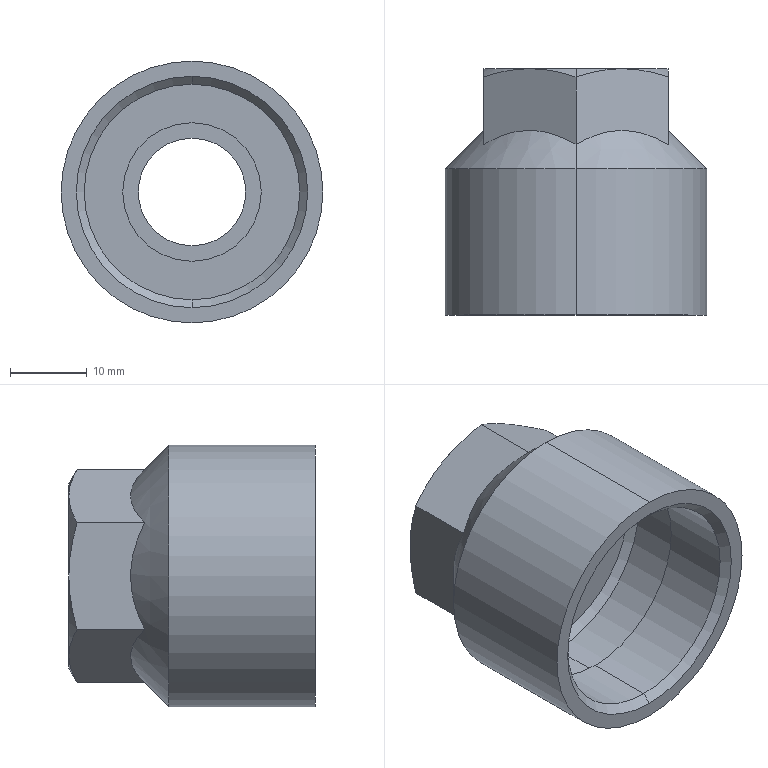Part | SolidWorks | features ICE 6, Chamfer 2, Extrusion 1, HoleWzd 1 | 1 solid | 36 faces | box 34 x 32 x 34 mm | volume 9791 mm3 | cone 15 | plane 11 | cylinder 10 | commonest cylinder face diameters 14 x2 18 x2 28 x2 30 x2 34 x2
STEP:
#1=CARTESIAN_POINT('',(0.,8.,12.));
#2=VERTEX_POINT('',#1);
#3=CARTESIAN_POINT('',(6.,8.,10.392));
#4=VERTEX_POINT('',#3);
#5=CARTESIAN_POINT('',(0.,8.,0.));
#6=DIRECTION('',(0.,1.,0.));
#7=DIRECTION('',(0.,0.,1.));
#8=AXIS2_PLACEMENT_3D('',#5,#6,#7);
#9=CIRCLE('',#8,12.);
#10=EDGE_CURVE('',#2,#4,#9,.T.);
#11=ORIENTED_EDGE('',*,*,#10,.F.);
#12=CARTESIAN_POINT('',(0.,6.928,13.856));
#13=VERTEX_POINT('',#12);
#14=CARTESIAN_POINT('',(0.,8.,12.));
#15=DIRECTION('',(0.,-0.5,0.866));
#16=VECTOR('',#15,1000.);
#17=LINE('',#14,#16);
#18=EDGE_CURVE('',#2,#13,#17,.T.);
#19=ORIENTED_EDGE('',*,*,#18,.T.);
#20=CARTESIAN_POINT('',(0.,6.928,13.856));
#21=CARTESIAN_POINT('',(0.9815,7.255,13.29));
#22=CARTESIAN_POINT('',(1.97,7.525,12.719));
#23=CARTESIAN_POINT('',(3.968,7.898,11.565));
#24=CARTESIAN_POINT('',(4.978,8.,10.982));
#25=CARTESIAN_POINT('',(6.,8.,10.392));
#26=B_SPLINE_CURVE_WITH_KNOTS('',3,(#20,#21,#22,#23,#24,#25),.UNSPECIFIED.,.F.,.F.,(4,2,4),(0.000000238,0.003505,0.00701),.UNSPECIFIED.);
#27=EDGE_CURVE('',#13,#4,#26,.T.);
#28=ORIENTED_EDGE('',*,*,#27,.T.);
#29=EDGE_LOOP('',(#11,#19,#28));
#30=FACE_OUTER_BOUND('',#29,.T.);
#31=CARTESIAN_POINT('',(0.,8.,0.));
#32=DIRECTION('',(0.,-1.,0.));
#33=DIRECTION('',(0.,0.,1.));
#34=AXIS2_PLACEMENT_3D('',#31,#32,#33);
#35=CONICAL_SURFACE('',#34,12.,1.047);
#36=ADVANCED_FACE('',(#30),#35,.T.);
#37=CARTESIAN_POINT('',(0.,-1.856,13.856));
#38=VERTEX_POINT('',#37);
#39=CARTESIAN_POINT('',(12.,-1.856,6.928));
#40=VERTEX_POINT('',#39);
#41=CARTESIAN_POINT('',(0.,-1.856,13.856));
#42=CARTESIAN_POINT('',(0.9376,-1.315,13.315));
#43=CARTESIAN_POINT('',(1.896,-0.8548,12.762));
#44=CARTESIAN_POINT('',(3.386,-0.3616,11.902));
#45=CARTESIAN_POINT('',(3.891,-0.2304,11.61));
#46=CARTESIAN_POINT('',(4.923,-0.04992,11.014));
#47=CARTESIAN_POINT('',(5.454,-0.001312,10.707));
#48=CARTESIAN_POINT('',(7.025,0.002543,9.8));
#49=CARTESIAN_POINT('',(8.055,-0.1806,9.206));
#50=CARTESIAN_POINT('',(10.086,-0.845,8.033));
#51=CARTESIAN_POINT('',(11.057,-1.312,7.473));
#52=CARTESIAN_POINT('',(12.,-1.856,6.928));
#53=B_SPLINE_CURVE_WITH_KNOTS('',3,(#41,#42,#43,#44,#45,#46,#47,#48,#49,#50,#51,#52),.UNSPECIFIED.,.F.,.F.,(4,2,2,2,2,4),(0.,0.003578,0.005367,0.007157,0.01073,0.01431),.UNSPECIFIED.);
#54=EDGE_CURVE('',#38,#40,#53,.T.);
#55=ORIENTED_EDGE('',*,*,#54,.F.);
#56=CARTESIAN_POINT('',(0.,-5.,17.));
#57=VERTEX_POINT('',#56);
#58=CARTESIAN_POINT('',(0.,-5.,17.));
#59=DIRECTION('',(0.,-0.7071,0.7071));
#60=VECTOR('',#59,1000.);
#61=LINE('',#58,#60);
#62=EDGE_CURVE('',#38,#57,#61,.T.);
#63=ORIENTED_EDGE('',*,*,#62,.T.);
#64=CARTESIAN_POINT('',(0.,-5.,-17.));
#65=VERTEX_POINT('',#64);
#66=CARTESIAN_POINT('',(0.,-5.,0.));
#67=DIRECTION('',(0.,-1.,0.));
#68=DIRECTION('',(0.,0.,-1.));
#69=AXIS2_PLACEMENT_3D('',#66,#67,#68);
#70=CIRCLE('',#69,17.);
#71=EDGE_CURVE('',#65,#57,#70,.T.);
#72=ORIENTED_EDGE('',*,*,#71,.F.);
#73=CARTESIAN_POINT('',(0.,-1.856,-13.856));
#74=VERTEX_POINT('',#73);
#75=CARTESIAN_POINT('',(0.,-5.,-17.));
#76=DIRECTION('',(0.,-0.7071,-0.7071));
#77=VECTOR('',#76,1000.);
#78=LINE('',#75,#77);
#79=EDGE_CURVE('',#74,#65,#78,.T.);
#80=ORIENTED_EDGE('',*,*,#79,.F.);
#81=CARTESIAN_POINT('',(12.,-1.856,-6.928));
#82=VERTEX_POINT('',#81);
#83=CARTESIAN_POINT('',(12.,-1.856,-6.928));
#84=CARTESIAN_POINT('',(11.062,-1.315,-7.47));
#85=CARTESIAN_POINT('',(10.104,-0.8548,-8.023));
#86=CARTESIAN_POINT('',(8.614,-0.3616,-8.883));
#87=CARTESIAN_POINT('',(8.109,-0.2304,-9.175));
#88=CARTESIAN_POINT('',(7.077,-0.04992,-9.77));
#89=CARTESIAN_POINT('',(6.546,-0.001312,-10.077));
#90=CARTESIAN_POINT('',(4.975,0.002543,-10.984));
#91=CARTESIAN_POINT('',(3.945,-0.1806,-11.579));
#92=CARTESIAN_POINT('',(1.914,-0.845,-12.751));
#93=CARTESIAN_POINT('',(0.9431,-1.312,-13.312));
#94=CARTESIAN_POINT('',(0.,-1.856,-13.856));
#95=B_SPLINE_CURVE_WITH_KNOTS('',3,(#83,#84,#85,#86,#87,#88,#89,#90,#91,#92,#93,#94),.UNSPECIFIED.,.F.,.F.,(4,2,2,2,2,4),(0.,0.003578,0.005367,0.007157,0.01073,0.01431),.UNSPECIFIED.);
#96=EDGE_CURVE('',#82,#74,#95,.T.);
#97=ORIENTED_EDGE('',*,*,#96,.F.);
#98=CARTESIAN_POINT('',(12.,-1.856,6.928));
#99=CARTESIAN_POINT('',(12.,-1.315,5.846));
#100=CARTESIAN_POINT('',(12.,-0.8548,4.739));
#101=CARTESIAN_POINT('',(12.,-0.3616,3.019));
#102=CARTESIAN_POINT('',(12.,-0.2304,2.435));
#103=CARTESIAN_POINT('',(12.,-0.04992,1.244));
#104=CARTESIAN_POINT('',(12.,-0.001312,0.6303));
#105=CARTESIAN_POINT('',(12.,0.002543,-1.184));
#106=CARTESIAN_POINT('',(12.,-0.1806,-2.373));
#107=CARTESIAN_POINT('',(12.,-0.845,-4.718));
#108=CARTESIAN_POINT('',(12.,-1.312,-5.839));
#109=CARTESIAN_POINT('',(12.,-1.856,-6.928));
#110=B_SPLINE_CURVE_WITH_KNOTS('',3,(#98,#99,#100,#101,#102,#103,#104,#105,#106,#107,#108,#109),.UNSPECIFIED.,.F.,.F.,(4,2,2,2,2,4),(0.,0.003578,0.005367,0.007157,0.01073,0.01431),.UNSPECIFIED.);
#111=EDGE_CURVE('',#40,#82,#110,.T.);
#112=ORIENTED_EDGE('',*,*,#111,.F.);
#113=EDGE_LOOP('',(#55,#63,#72,#80,#97,#112));
#114=FACE_OUTER_BOUND('',#113,.T.);
#115=CARTESIAN_POINT('',(0.,-5.,0.));
#116=DIRECTION('',(0.,-1.,0.));
#117=DIRECTION('',(0.,0.,-1.));
#118=AXIS2_PLACEMENT_3D('',#115,#116,#117);
#119=CONICAL_SURFACE('',#118,17.,0.7854);
#120=ADVANCED_FACE('',(#114),#119,.T.);
#121=CARTESIAN_POINT('',(0.,7.,-7.));
#122=VERTEX_POINT('',#121);
#123=CARTESIAN_POINT('',(0.,7.,7.));
#124=VERTEX_POINT('',#123);
#125=CARTESIAN_POINT('',(0.,7.,0.));
#126=DIRECTION('',(0.,1.,0.));
#127=DIRECTION('',(0.,0.,1.));
#128=AXIS2_PLACEMENT_3D('',#125,#126,#127);
#129=CIRCLE('',#128,7.);
#130=EDGE_CURVE('',#122,#124,#129,.T.);
#131=ORIENTED_EDGE('',*,*,#130,.F.);
#132=CARTESIAN_POINT('',(0.,8.,-8.));
#133=VERTEX_POINT('',#132);
#134=CARTESIAN_POINT('',(0.,7.,-7.));
#135=DIRECTION('',(0.,0.7071,-0.7071));
#136=VECTOR('',#135,1000.);
#137=LINE('',#134,#136);
#138=EDGE_CURVE('',#122,#133,#137,.T.);
#139=ORIENTED_EDGE('',*,*,#138,.T.);
#140=CARTESIAN_POINT('',(0.,8.,8.));
#141=VERTEX_POINT('',#140);
#142=CARTESIAN_POINT('',(0.,8.,0.));
#143=DIRECTION('',(0.,-1.,0.));
#144=DIRECTION('',(0.,0.,1.));
#145=AXIS2_PLACEMENT_3D('',#142,#143,#144);
#146=CIRCLE('',#145,8.);
#147=EDGE_CURVE('',#141,#133,#146,.T.);
#148=ORIENTED_EDGE('',*,*,#147,.F.);
#149=CARTESIAN_POINT('',(0.,7.,7.));
#150=DIRECTION('',(0.,0.7071,0.7071));
#151=VECTOR('',#150,1000.);
#152=LINE('',#149,#151);
#153=EDGE_CURVE('',#124,#141,#152,.T.);
#154=ORIENTED_EDGE('',*,*,#153,.F.);
#155=EDGE_LOOP('',(#131,#139,#148,#154));
#156=FACE_OUTER_BOUND('',#155,.T.);
#157=CARTESIAN_POINT('',(0.,7.,0.));
#158=DIRECTION('',(0.,1.,0.));
#159=DIRECTION('',(0.,0.,1.));
#160=AXIS2_PLACEMENT_3D('',#157,#158,#159);
#161=CONICAL_SURFACE('',#160,7.,0.7854);
#162=ADVANCED_FACE('',(#156),#161,.F.);
#163=CARTESIAN_POINT('',(0.,-6.,-14.));
#164=VERTEX_POINT('',#163);
#165=CARTESIAN_POINT('',(0.,-6.,14.));
#166=VERTEX_POINT('',#165);
#167=CARTESIAN_POINT('',(0.,-6.,0.));
#168=DIRECTION('',(0.,1.,0.));
#169=DIRECTION('',(0.,0.,1.));
#170=AXIS2_PLACEMENT_3D('',#167,#168,#169);
#171=CIRCLE('',#170,14.);
#172=EDGE_CURVE('',#164,#166,#171,.T.);
#173=ORIENTED_EDGE('',*,*,#172,.T.);
#174=CARTESIAN_POINT('',(0.,-7.,15.));
#175=VERTEX_POINT('',#174);
#176=CARTESIAN_POINT('',(0.,-7.,15.));
#177=DIRECTION('',(0.,-0.7071,0.7071));
#178=VECTOR('',#177,1000.);
#179=LINE('',#176,#178);
#180=EDGE_CURVE('',#166,#175,#179,.T.);
#181=ORIENTED_EDGE('',*,*,#180,.T.);
#182=CARTESIAN_POINT('',(0.,-7.,-15.));
#183=VERTEX_POINT('',#182);
#184=CARTESIAN_POINT('',(0.,-7.,0.));
#185=DIRECTION('',(0.,1.,0.));
#186=DIRECTION('',(0.,0.,1.));
#187=AXIS2_PLACEMENT_3D('',#184,#185,#186);
#188=CIRCLE('',#187,15.);
#189=EDGE_CURVE('',#183,#175,#188,.T.);
#190=ORIENTED_EDGE('',*,*,#189,.F.);
#191=CARTESIAN_POINT('',(0.,-7.,-15.));
#192=DIRECTION('',(0.,-0.7071,-0.7071));
#193=VECTOR('',#192,1000.);
#194=LINE('',#191,#193);
#195=EDGE_CURVE('',#164,#183,#194,.T.);
#196=ORIENTED_EDGE('',*,*,#195,.F.);
#197=EDGE_LOOP('',(#173,#181,#190,#196));
#198=FACE_OUTER_BOUND('',#197,.T.);
#199=CARTESIAN_POINT('',(0.,-7.,0.));
#200=DIRECTION('',(0.,-1.,0.));
#201=DIRECTION('',(0.,0.,-1.));
#202=AXIS2_PLACEMENT_3D('',#199,#200,#201);
#203=CONICAL_SURFACE('',#202,15.,0.7854);
#204=ADVANCED_FACE('',(#198),#203,.F.);
#205=CARTESIAN_POINT('',(0.,-22.975,14.));
#206=VERTEX_POINT('',#205);
#207=CARTESIAN_POINT('',(0.,-22.975,-14.));
#208=VERTEX_POINT('',#207);
#209=CARTESIAN_POINT('',(0.,-22.975,0.));
#210=DIRECTION('',(0.,-1.,0.));
#211=DIRECTION('',(0.,0.,-1.));
#212=AXIS2_PLACEMENT_3D('',#209,#210,#211);
#213=CIRCLE('',#212,14.);
#214=EDGE_CURVE('',#206,#208,#213,.T.);
#215=ORIENTED_EDGE('',*,*,#214,.F.);
#216=CARTESIAN_POINT('',(0.,-24.,15.025));
#217=VERTEX_POINT('',#216);
#218=CARTESIAN_POINT('',(0.,-24.,15.025));
#219=DIRECTION('',(0.,-0.7071,0.7071));
#220=VECTOR('',#219,1000.);
#221=LINE('',#218,#220);
#222=EDGE_CURVE('',#206,#217,#221,.T.);
#223=ORIENTED_EDGE('',*,*,#222,.T.);
#224=CARTESIAN_POINT('',(0.,-24.,-15.025));
#225=VERTEX_POINT('',#224);
#226=CARTESIAN_POINT('',(0.,-24.,0.));
#227=DIRECTION('',(0.,-1.,0.));
#228=DIRECTION('',(0.,0.,-1.));
#229=AXIS2_PLACEMENT_3D('',#226,#227,#228);
#230=CIRCLE('',#229,15.025);
#231=EDGE_CURVE('',#217,#225,#230,.T.);
#232=ORIENTED_EDGE('',*,*,#231,.T.);
#233=CARTESIAN_POINT('',(0.,-24.,-15.025));
#234=DIRECTION('',(0.,-0.7071,-0.7071));
#235=VECTOR('',#234,1000.);
#236=LINE('',#233,#235);
#237=EDGE_CURVE('',#208,#225,#236,.T.);
#238=ORIENTED_EDGE('',*,*,#237,.F.);
#239=EDGE_LOOP('',(#215,#223,#232,#238));
#240=FACE_OUTER_BOUND('',#239,.T.);
#241=CARTESIAN_POINT('',(0.,-24.,0.));
#242=DIRECTION('',(0.,-1.,0.));
#243=DIRECTION('',(0.,0.,-1.));
#244=AXIS2_PLACEMENT_3D('',#241,#242,#243);
#245=CONICAL_SURFACE('',#244,15.025,0.7854);
#246=ADVANCED_FACE('',(#240),#245,.F.);
#247=CARTESIAN_POINT('',(0.,-14.,14.));
#248=VERTEX_POINT('',#247);
#249=CARTESIAN_POINT('',(0.,-14.,-14.));
#250=VERTEX_POINT('',#249);
#251=CARTESIAN_POINT('',(0.,-14.,0.));
#252=DIRECTION('',(0.,-1.,0.));
#253=DIRECTION('',(0.,0.,-1.));
#254=AXIS2_PLACEMENT_3D('',#251,#252,#253);
#255=CIRCLE('',#254,14.);
#256=EDGE_CURVE('',#248,#250,#255,.T.);
#257=ORIENTED_EDGE('',*,*,#256,.F.);
#258=CARTESIAN_POINT('',(0.,-24.,14.));
#259=DIRECTION('',(0.,-1.,0.));
#260=VECTOR('',#259,1000.);
#261=LINE('',#258,#260);
#262=EDGE_CURVE('',#248,#206,#261,.T.);
#263=ORIENTED_EDGE('',*,*,#262,.T.);
#264=ORIENTED_EDGE('',*,*,#214,.T.);
#265=CARTESIAN_POINT('',(0.,-24.,-14.));
#266=DIRECTION('',(0.,-1.,0.));
#267=VECTOR('',#266,1000.);
#268=LINE('',#265,#267);
#269=EDGE_CURVE('',#250,#208,#268,.T.);
#270=ORIENTED_EDGE('',*,*,#269,.F.);
#271=EDGE_LOOP('',(#257,#263,#264,#270));
#272=FACE_OUTER_BOUND('',#271,.T.);
#273=CARTESIAN_POINT('',(0.,-24.,0.));
#274=DIRECTION('',(0.,-1.,0.));
#275=DIRECTION('',(0.,0.,-1.));
#276=AXIS2_PLACEMENT_3D('',#273,#274,#275);
#277=CYLINDRICAL_SURFACE('',#276,14.);
#278=ADVANCED_FACE('',(#272),#277,.F.);
#279=CARTESIAN_POINT('',(0.,-14.,-15.));
#280=VERTEX_POINT('',#279);
#281=CARTESIAN_POINT('',(0.,-14.,15.));
#282=VERTEX_POINT('',#281);
#283=CARTESIAN_POINT('',(0.,-14.,0.));
#284=DIRECTION('',(0.,1.,0.));
#285=DIRECTION('',(0.,0.,1.));
#286=AXIS2_PLACEMENT_3D('',#283,#284,#285);
#287=CIRCLE('',#286,15.);
#288=EDGE_CURVE('',#280,#282,#287,.T.);
#289=ORIENTED_EDGE('',*,*,#288,.F.);
#290=CARTESIAN_POINT('',(0.,-14.,-15.));
#291=DIRECTION('',(0.,1.,0.));
#292=VECTOR('',#291,1000.);
#293=LINE('',#290,#292);
#294=EDGE_CURVE('',#280,#183,#293,.T.);
#295=ORIENTED_EDGE('',*,*,#294,.T.);
#296=ORIENTED_EDGE('',*,*,#189,.T.);
#297=CARTESIAN_POINT('',(0.,-14.,15.));
#298=DIRECTION('',(0.,1.,0.));
#299=VECTOR('',#298,1000.);
#300=LINE('',#297,#299);
#301=EDGE_CURVE('',#282,#175,#300,.T.);
#302=ORIENTED_EDGE('',*,*,#301,.F.);
#303=EDGE_LOOP('',(#289,#295,#296,#302));
#304=FACE_OUTER_BOUND('',#303,.T.);
#305=CARTESIAN_POINT('',(0.,-14.,0.));
#306=DIRECTION('',(0.,1.,0.));
#307=DIRECTION('',(0.,0.,1.));
#308=AXIS2_PLACEMENT_3D('',#305,#306,#307);
#309=CYLINDRICAL_SURFACE('',#308,15.);
#310=ADVANCED_FACE('',(#304),#309,.F.);
#311=CARTESIAN_POINT('',(0.,-6.,-9.));
#312=VERTEX_POINT('',#311);
#313=CARTESIAN_POINT('',(0.,-6.,9.));
#314=VERTEX_POINT('',#313);
#315=CARTESIAN_POINT('',(0.,-6.,0.));
#316=DIRECTION('',(0.,1.,0.));
#317=DIRECTION('',(0.,0.,1.));
#318=AXIS2_PLACEMENT_3D('',#315,#316,#317);
#319=CIRCLE('',#318,9.);
#320=EDGE_CURVE('',#312,#314,#319,.T.);
#321=ORIENTED_EDGE('',*,*,#320,.F.);
#322=CARTESIAN_POINT('',(0.,2.,-9.));
#323=VERTEX_POINT('',#322);
#324=CARTESIAN_POINT('',(0.,-6.,-9.));
#325=DIRECTION('',(0.,1.,0.));
#326=VECTOR('',#325,1000.);
#327=LINE('',#324,#326);
#328=EDGE_CURVE('',#312,#323,#327,.T.);
#329=ORIENTED_EDGE('',*,*,#328,.T.);
#330=CARTESIAN_POINT('',(0.,2.,9.));
#331=VERTEX_POINT('',#330);
#332=CARTESIAN_POINT('',(0.,2.,0.));
#333=DIRECTION('',(0.,1.,0.));
#334=DIRECTION('',(0.,0.,1.));
#335=AXIS2_PLACEMENT_3D('',#332,#333,#334);
#336=CIRCLE('',#335,9.);
#337=EDGE_CURVE('',#323,#331,#336,.T.);
#338=ORIENTED_EDGE('',*,*,#337,.T.);
#339=CARTESIAN_POINT('',(0.,-6.,9.));
#340=DIRECTION('',(0.,1.,0.));
#341=VECTOR('',#340,1000.);
#342=LINE('',#339,#341);
#343=EDGE_CURVE('',#314,#331,#342,.T.);
#344=ORIENTED_EDGE('',*,*,#343,.F.);
#345=EDGE_LOOP('',(#321,#329,#338,#344));
#346=FACE_OUTER_BOUND('',#345,.T.);
#347=CARTESIAN_POINT('',(0.,-6.,0.));
#348=DIRECTION('',(0.,1.,0.));
#349=DIRECTION('',(0.,0.,1.));
#350=AXIS2_PLACEMENT_3D('',#347,#348,#349);
#351=CYLINDRICAL_SURFACE('',#350,9.);
#352=ADVANCED_FACE('',(#346),#351,.F.);
#353=CARTESIAN_POINT('',(0.,2.,-7.));
#354=VERTEX_POINT('',#353);
#355=CARTESIAN_POINT('',(0.,2.,7.));
#356=VERTEX_POINT('',#355);
#357=CARTESIAN_POINT('',(0.,2.,0.));
#358=DIRECTION('',(0.,1.,0.));
#359=DIRECTION('',(0.,0.,1.));
#360=AXIS2_PLACEMENT_3D('',#357,#358,#359);
#361=CIRCLE('',#360,7.);
#362=EDGE_CURVE('',#354,#356,#361,.T.);
#363=ORIENTED_EDGE('',*,*,#362,.F.);
#364=CARTESIAN_POINT('',(0.,2.,-7.));
#365=DIRECTION('',(0.,1.,0.));
#366=VECTOR('',#365,1000.);
#367=LINE('',#364,#366);
#368=EDGE_CURVE('',#354,#122,#367,.T.);
#369=ORIENTED_EDGE('',*,*,#368,.T.);
#370=ORIENTED_EDGE('',*,*,#130,.T.);
#371=CARTESIAN_POINT('',(0.,2.,7.));
#372=DIRECTION('',(0.,1.,0.));
#373=VECTOR('',#372,1000.);
#374=LINE('',#371,#373);
#375=EDGE_CURVE('',#356,#124,#374,.T.);
#376=ORIENTED_EDGE('',*,*,#375,.F.);
#377=EDGE_LOOP('',(#363,#369,#370,#376));
#378=FACE_OUTER_BOUND('',#377,.T.);
#379=CARTESIAN_POINT('',(0.,2.,0.));
#380=DIRECTION('',(0.,1.,0.));
#381=DIRECTION('',(0.,0.,1.));
#382=AXIS2_PLACEMENT_3D('',#379,#380,#381);
#383=CYLINDRICAL_SURFACE('',#382,7.);
#384=ADVANCED_FACE('',(#378),#383,.F.);
#385=CARTESIAN_POINT('',(0.,-24.,-17.));
#386=VERTEX_POINT('',#385);
#387=CARTESIAN_POINT('',(0.,-24.,17.));
#388=VERTEX_POINT('',#387);
#389=CARTESIAN_POINT('',(0.,-24.,0.));
#390=DIRECTION('',(0.,-1.,0.));
#391=DIRECTION('',(0.,0.,-1.));
#392=AXIS2_PLACEMENT_3D('',#389,#390,#391);
#393=CIRCLE('',#392,17.);
#394=EDGE_CURVE('',#386,#388,#393,.T.);
#395=ORIENTED_EDGE('',*,*,#394,.F.);
#396=CARTESIAN_POINT('',(0.,-24.,-17.));
#397=DIRECTION('',(0.,1.,0.));
#398=VECTOR('',#397,1000.);
#399=LINE('',#396,#398);
#400=EDGE_CURVE('',#386,#65,#399,.T.);
#401=ORIENTED_EDGE('',*,*,#400,.T.);
#402=ORIENTED_EDGE('',*,*,#71,.T.);
#403=CARTESIAN_POINT('',(0.,-24.,17.));
#404=DIRECTION('',(0.,1.,0.));
#405=VECTOR('',#404,1000.);
#406=LINE('',#403,#405);
#407=EDGE_CURVE('',#388,#57,#406,.T.);
#408=ORIENTED_EDGE('',*,*,#407,.F.);
#409=EDGE_LOOP('',(#395,#401,#402,#408));
#410=FACE_OUTER_BOUND('',#409,.T.);
#411=CARTESIAN_POINT('',(0.,-24.,0.));
#412=DIRECTION('',(0.,1.,0.));
#413=DIRECTION('',(0.,0.,1.));
#414=AXIS2_PLACEMENT_3D('',#411,#412,#413);
#415=CYLINDRICAL_SURFACE('',#414,17.);
#416=ADVANCED_FACE('',(#410),#415,.T.);
#417=CARTESIAN_POINT('',(12.,6.928,-6.928));
#418=VERTEX_POINT('',#417);
#419=CARTESIAN_POINT('',(6.,8.,-10.392));
#420=VERTEX_POINT('',#419);
#421=CARTESIAN_POINT('',(12.,6.928,-6.928));
#422=CARTESIAN_POINT('',(11.018,7.255,-7.495));
#423=CARTESIAN_POINT('',(10.03,7.525,-8.066));
#424=CARTESIAN_POINT('',(8.032,7.898,-9.219));
#425=CARTESIAN_POINT('',(7.022,8.,-9.802));
#426=CARTESIAN_POINT('',(6.,8.,-10.392));
#427=B_SPLINE_CURVE_WITH_KNOTS('',3,(#421,#422,#423,#424,#425,#426),.UNSPECIFIED.,.F.,.F.,(4,2,4),(0.000000238,0.003505,0.00701),.UNSPECIFIED.);
#428=EDGE_CURVE('',#418,#420,#427,.T.);
#429=ORIENTED_EDGE('',*,*,#428,.F.);
#430=CARTESIAN_POINT('',(12.,8.,-6.928));
#431=DIRECTION('',(0.,-1.,0.));
#432=VECTOR('',#431,1000.);
#433=LINE('',#430,#432);
#434=EDGE_CURVE('',#418,#82,#433,.T.);
#435=ORIENTED_EDGE('',*,*,#434,.T.);
#436=ORIENTED_EDGE('',*,*,#96,.T.);
#437=CARTESIAN_POINT('',(0.,6.928,-13.856));
#438=VERTEX_POINT('',#437);
#439=CARTESIAN_POINT('',(0.,8.,-13.856));
#440=DIRECTION('',(0.,-1.,0.));
#441=VECTOR('',#440,1000.);
#442=LINE('',#439,#441);
#443=EDGE_CURVE('',#438,#74,#442,.T.);
#444=ORIENTED_EDGE('',*,*,#443,.F.);
#445=CARTESIAN_POINT('',(6.,8.,-10.392));
#446=CARTESIAN_POINT('',(5.491,8.,-10.686));
#447=CARTESIAN_POINT('',(4.979,7.975,-10.982));
#448=CARTESIAN_POINT('',(3.967,7.877,-11.566));
#449=CARTESIAN_POINT('',(3.465,7.804,-11.856));
#450=CARTESIAN_POINT('',(1.966,7.524,-12.721));
#451=CARTESIAN_POINT('',(0.9791,7.255,-13.291));
#452=CARTESIAN_POINT('',(0.,6.928,-13.856));
#453=B_SPLINE_CURVE_WITH_KNOTS('',3,(#445,#446,#447,#448,#449,#450,#451,#452),.UNSPECIFIED.,.F.,.F.,(4,2,2,4),(0.00701,0.008756,0.0105,0.01399),.UNSPECIFIED.);
#454=EDGE_CURVE('',#420,#438,#453,.T.);
#455=ORIENTED_EDGE('',*,*,#454,.F.);
#456=EDGE_LOOP('',(#429,#435,#436,#444,#455));
#457=FACE_OUTER_BOUND('',#456,.T.);
#458=CARTESIAN_POINT('',(12.,8.,-6.928));
#459=DIRECTION('',(-0.5,0.,0.866));
#460=DIRECTION('',(0.866,0.,0.5));
#461=AXIS2_PLACEMENT_3D('',#458,#459,#460);
#462=PLANE('',#461);
#463=ADVANCED_FACE('',(#457),#462,.F.);
#464=CARTESIAN_POINT('',(-6.,8.,-10.392));
#465=VERTEX_POINT('',#464);
#466=CARTESIAN_POINT('',(0.,6.928,-13.856));
#467=CARTESIAN_POINT('',(-0.9815,7.255,-13.29));
#468=CARTESIAN_POINT('',(-1.97,7.525,-12.719));
#469=CARTESIAN_POINT('',(-3.968,7.898,-11.565));
#470=CARTESIAN_POINT('',(-4.978,8.,-10.982));
#471=CARTESIAN_POINT('',(-6.,8.,-10.392));
#472=B_SPLINE_CURVE_WITH_KNOTS('',3,(#466,#467,#468,#469,#470,#471),.UNSPECIFIED.,.F.,.F.,(4,2,4),(0.000000238,0.003505,0.00701),.UNSPECIFIED.);
#473=EDGE_CURVE('',#438,#465,#472,.T.);
#474=ORIENTED_EDGE('',*,*,#473,.F.);
#475=ORIENTED_EDGE('',*,*,#443,.T.);
#476=CARTESIAN_POINT('',(-12.,-1.856,-6.928));
#477=VERTEX_POINT('',#476);
#478=CARTESIAN_POINT('',(0.,-1.856,-13.856));
#479=CARTESIAN_POINT('',(-0.9376,-1.315,-13.315));
#480=CARTESIAN_POINT('',(-1.896,-0.8549,-12.762));
#481=CARTESIAN_POINT('',(-3.386,-0.3617,-11.902));
#482=CARTESIAN_POINT('',(-3.891,-0.2305,-11.61));
#483=CARTESIAN_POINT('',(-4.923,-0.04994,-11.014));
#484=CARTESIAN_POINT('',(-5.454,-0.001324,-10.708));
#485=CARTESIAN_POINT('',(-7.025,0.002566,-9.8));
#486=CARTESIAN_POINT('',(-8.055,-0.1806,-9.206));
#487=CARTESIAN_POINT('',(-10.086,-0.8452,-8.033));
#488=CARTESIAN_POINT('',(-11.057,-1.312,-7.473));
#489=CARTESIAN_POINT('',(-12.,-1.856,-6.928));
#490=B_SPLINE_CURVE_WITH_KNOTS('',3,(#478,#479,#480,#481,#482,#483,#484,#485,#486,#487,#488,#489),.UNSPECIFIED.,.F.,.F.,(4,2,2,2,2,4),(-0.01096,-0.007318,-0.005498,-0.003678,-0.00003841,0.003601),.UNSPECIFIED.);
#491=EDGE_CURVE('',#74,#477,#490,.T.);
#492=ORIENTED_EDGE('',*,*,#491,.T.);
#493=CARTESIAN_POINT('',(-12.,6.928,-6.928));
#494=VERTEX_POINT('',#493);
#495=CARTESIAN_POINT('',(-12.,8.,-6.928));
#496=DIRECTION('',(0.,-1.,0.));
#497=VECTOR('',#496,1000.);
#498=LINE('',#495,#497);
#499=EDGE_CURVE('',#494,#477,#498,.T.);
#500=ORIENTED_EDGE('',*,*,#499,.F.);
#501=CARTESIAN_POINT('',(-6.,8.,-10.392));
#502=CARTESIAN_POINT('',(-6.509,8.,-10.098));
#503=CARTESIAN_POINT('',(-7.021,7.975,-9.803));
#504=CARTESIAN_POINT('',(-8.033,7.877,-9.219));
#505=CARTESIAN_POINT('',(-8.535,7.804,-8.929));
#506=CARTESIAN_POINT('',(-10.034,7.524,-8.063));
#507=CARTESIAN_POINT('',(-11.021,7.255,-7.493));
#508=CARTESIAN_POINT('',(-12.,6.928,-6.928));
#509=B_SPLINE_CURVE_WITH_KNOTS('',3,(#501,#502,#503,#504,#505,#506,#507,#508),.UNSPECIFIED.,.F.,.F.,(4,2,2,4),(0.00701,0.008756,0.0105,0.01399),.UNSPECIFIED.);
#510=EDGE_CURVE('',#465,#494,#509,.T.);
#511=ORIENTED_EDGE('',*,*,#510,.F.);
#512=EDGE_LOOP('',(#474,#475,#492,#500,#511));
#513=FACE_OUTER_BOUND('',#512,.T.);
#514=CARTESIAN_POINT('',(0.,8.,-13.856));
#515=DIRECTION('',(0.5,0.,0.866));
#516=DIRECTION('',(0.866,0.,-0.5));
#517=AXIS2_PLACEMENT_3D('',#514,#515,#516);
#518=PLANE('',#517);
#519=ADVANCED_FACE('',(#513),#518,.F.);
#520=CARTESIAN_POINT('',(-12.,8.,0.));
#521=VERTEX_POINT('',#520);
#522=CARTESIAN_POINT('',(-12.,6.928,-6.928));
#523=CARTESIAN_POINT('',(-12.,7.254,-5.8));
#524=CARTESIAN_POINT('',(-12.,7.523,-4.662));
#525=CARTESIAN_POINT('',(-12.,7.897,-2.356));
#526=CARTESIAN_POINT('',(-12.,8.,-1.187));
#527=CARTESIAN_POINT('',(-12.,8.,0.));
#528=B_SPLINE_CURVE_WITH_KNOTS('',3,(#522,#523,#524,#525,#526,#527),.UNSPECIFIED.,.F.,.F.,(4,2,4),(0.01541,0.01893,0.02245),.UNSPECIFIED.);
#529=EDGE_CURVE('',#494,#521,#528,.T.);
#530=ORIENTED_EDGE('',*,*,#529,.F.);
#531=ORIENTED_EDGE('',*,*,#499,.T.);
#532=CARTESIAN_POINT('',(-12.,-1.856,6.928));
#533=VERTEX_POINT('',#532);
#534=CARTESIAN_POINT('',(-12.,-1.856,-6.928));
#535=CARTESIAN_POINT('',(-12.,-1.315,-5.846));
#536=CARTESIAN_POINT('',(-12.,-0.8548,-4.739));
#537=CARTESIAN_POINT('',(-12.,-0.3616,-3.019));
#538=CARTESIAN_POINT('',(-12.,-0.2304,-2.435));
#539=CARTESIAN_POINT('',(-12.,-0.04992,-1.244));
#540=CARTESIAN_POINT('',(-12.,-0.001312,-0.6303));
#541=CARTESIAN_POINT('',(-12.,0.002543,1.184));
#542=CARTESIAN_POINT('',(-12.,-0.1806,2.373));
#543=CARTESIAN_POINT('',(-12.,-0.845,4.718));
#544=CARTESIAN_POINT('',(-12.,-1.312,5.839));
#545=CARTESIAN_POINT('',(-12.,-1.856,6.928));
#546=B_SPLINE_CURVE_WITH_KNOTS('',3,(#534,#535,#536,#537,#538,#539,#540,#541,#542,#543,#544,#545),.UNSPECIFIED.,.F.,.F.,(4,2,2,2,2,4),(0.,0.003578,0.005367,0.007157,0.01073,0.01431),.UNSPECIFIED.);
#547=EDGE_CURVE('',#477,#533,#546,.T.);
#548=ORIENTED_EDGE('',*,*,#547,.T.);
#549=CARTESIAN_POINT('',(-12.,6.928,6.928));
#550=VERTEX_POINT('',#549);
#551=CARTESIAN_POINT('',(-12.,8.,6.928));
#552=DIRECTION('',(0.,-1.,0.));
#553=VECTOR('',#552,1000.);
#554=LINE('',#551,#553);
#555=EDGE_CURVE('',#550,#533,#554,.T.);
#556=ORIENTED_EDGE('',*,*,#555,.F.);
#557=CARTESIAN_POINT('',(-12.,8.,0.));
#558=CARTESIAN_POINT('',(-12.,8.,1.187));
#559=CARTESIAN_POINT('',(-12.,7.897,2.356));
#560=CARTESIAN_POINT('',(-12.,7.523,4.662));
#561=CARTESIAN_POINT('',(-12.,7.254,5.8));
#562=CARTESIAN_POINT('',(-12.,6.928,6.928));
#563=B_SPLINE_CURVE_WITH_KNOTS('',3,(#557,#558,#559,#560,#561,#562),.UNSPECIFIED.,.F.,.F.,(4,2,4),(0.02245,0.02598,0.0295),.UNSPECIFIED.);
#564=EDGE_CURVE('',#521,#550,#563,.T.);
#565=ORIENTED_EDGE('',*,*,#564,.F.);
#566=EDGE_LOOP('',(#530,#531,#548,#556,#565));
#567=FACE_OUTER_BOUND('',#566,.T.);
#568=CARTESIAN_POINT('',(-12.,8.,-6.928));
#569=DIRECTION('',(1.,0.,0.));
#570=DIRECTION('',(0.,0.,-1.));
#571=AXIS2_PLACEMENT_3D('',#568,#569,#570);
#572=PLANE('',#571);
#573=ADVANCED_FACE('',(#567),#572,.F.);
#574=CARTESIAN_POINT('',(-6.,8.,10.392));
#575=VERTEX_POINT('',#574);
#576=CARTESIAN_POINT('',(-12.,6.928,6.928));
#577=CARTESIAN_POINT('',(-11.018,7.255,7.495));
#578=CARTESIAN_POINT('',(-10.03,7.525,8.066));
#579=CARTESIAN_POINT('',(-8.032,7.898,9.219));
#580=CARTESIAN_POINT('',(-7.022,8.,9.802));
#581=CARTESIAN_POINT('',(-6.,8.,10.392));
#582=B_SPLINE_CURVE_WITH_KNOTS('',3,(#576,#577,#578,#579,#580,#581),.UNSPECIFIED.,.F.,.F.,(4,2,4),(0.000000238,0.003505,0.00701),.UNSPECIFIED.);
#583=EDGE_CURVE('',#550,#575,#582,.T.);
#584=ORIENTED_EDGE('',*,*,#583,.F.);
#585=ORIENTED_EDGE('',*,*,#555,.T.);
#586=CARTESIAN_POINT('',(-12.,-1.856,6.928));
#587=CARTESIAN_POINT('',(-11.062,-1.315,7.47));
#588=CARTESIAN_POINT('',(-10.104,-0.8548,8.023));
#589=CARTESIAN_POINT('',(-8.614,-0.3616,8.883));
#590=CARTESIAN_POINT('',(-8.109,-0.2304,9.175));
#591=CARTESIAN_POINT('',(-7.077,-0.04992,9.77));
#592=CARTESIAN_POINT('',(-6.546,-0.001312,10.077));
#593=CARTESIAN_POINT('',(-4.975,0.002543,10.984));
#594=CARTESIAN_POINT('',(-3.945,-0.1806,11.579));
#595=CARTESIAN_POINT('',(-1.914,-0.845,12.751));
#596=CARTESIAN_POINT('',(-0.9431,-1.312,13.312));
#597=CARTESIAN_POINT('',(0.,-1.856,13.856));
#598=B_SPLINE_CURVE_WITH_KNOTS('',3,(#586,#587,#588,#589,#590,#591,#592,#593,#594,#595,#596,#597),.UNSPECIFIED.,.F.,.F.,(4,2,2,2,2,4),(0.,0.003578,0.005367,0.007157,0.01073,0.01431),.UNSPECIFIED.);
#599=EDGE_CURVE('',#533,#38,#598,.T.);
#600=ORIENTED_EDGE('',*,*,#599,.T.);
#601=CARTESIAN_POINT('',(0.,8.,13.856));
#602=DIRECTION('',(0.,-1.,0.));
#603=VECTOR('',#602,1000.);
#604=LINE('',#601,#603);
#605=EDGE_CURVE('',#13,#38,#604,.T.);
#606=ORIENTED_EDGE('',*,*,#605,.F.);
#607=CARTESIAN_POINT('',(-6.,8.,10.392));
#608=CARTESIAN_POINT('',(-5.491,8.,10.686));
#609=CARTESIAN_POINT('',(-4.979,7.975,10.982));
#610=CARTESIAN_POINT('',(-3.967,7.877,11.566));
#611=CARTESIAN_POINT('',(-3.465,7.804,11.856));
#612=CARTESIAN_POINT('',(-1.966,7.524,12.721));
#613=CARTESIAN_POINT('',(-0.9791,7.255,13.291));
#614=CARTESIAN_POINT('',(0.,6.928,13.856));
#615=B_SPLINE_CURVE_WITH_KNOTS('',3,(#607,#608,#609,#610,#611,#612,#613,#614),.UNSPECIFIED.,.F.,.F.,(4,2,2,4),(0.00701,0.008756,0.0105,0.01399),.UNSPECIFIED.);
#616=EDGE_CURVE('',#575,#13,#615,.T.);
#617=ORIENTED_EDGE('',*,*,#616,.F.);
#618=EDGE_LOOP('',(#584,#585,#600,#606,#617));
#619=FACE_OUTER_BOUND('',#618,.T.);
#620=CARTESIAN_POINT('',(-12.,8.,6.928));
#621=DIRECTION('',(0.5,0.,-0.866));
#622=DIRECTION('',(-0.866,0.,-0.5));
#623=AXIS2_PLACEMENT_3D('',#620,#621,#622);
#624=PLANE('',#623);
#625=ADVANCED_FACE('',(#619),#624,.F.);
#626=ORIENTED_EDGE('',*,*,#27,.F.);
#627=ORIENTED_EDGE('',*,*,#605,.T.);
#628=ORIENTED_EDGE('',*,*,#54,.T.);
#629=CARTESIAN_POINT('',(12.,6.928,6.928));
#630=VERTEX_POINT('',#629);
#631=CARTESIAN_POINT('',(12.,8.,6.928));
#632=DIRECTION('',(0.,-1.,0.));
#633=VECTOR('',#632,1000.);
#634=LINE('',#631,#633);
#635=EDGE_CURVE('',#630,#40,#634,.T.);
#636=ORIENTED_EDGE('',*,*,#635,.F.);
#637=CARTESIAN_POINT('',(6.,8.,10.392));
#638=CARTESIAN_POINT('',(6.509,8.,10.098));
#639=CARTESIAN_POINT('',(7.021,7.975,9.803));
#640=CARTESIAN_POINT('',(8.033,7.877,9.219));
#641=CARTESIAN_POINT('',(8.535,7.804,8.929));
#642=CARTESIAN_POINT('',(10.034,7.524,8.063));
#643=CARTESIAN_POINT('',(11.021,7.255,7.493));
#644=CARTESIAN_POINT('',(12.,6.928,6.928));
#645=B_SPLINE_CURVE_WITH_KNOTS('',3,(#637,#638,#639,#640,#641,#642,#643,#644),.UNSPECIFIED.,.F.,.F.,(4,2,2,4),(0.00701,0.008756,0.0105,0.01399),.UNSPECIFIED.);
#646=EDGE_CURVE('',#4,#630,#645,.T.);
#647=ORIENTED_EDGE('',*,*,#646,.F.);
#648=EDGE_LOOP('',(#626,#627,#628,#636,#647));
#649=FACE_OUTER_BOUND('',#648,.T.);
#650=CARTESIAN_POINT('',(0.,8.,13.856));
#651=DIRECTION('',(-0.5,0.,-0.866));
#652=DIRECTION('',(-0.866,0.,0.5));
#653=AXIS2_PLACEMENT_3D('',#650,#651,#652);
#654=PLANE('',#653);
#655=ADVANCED_FACE('',(#649),#654,.F.);
#656=CARTESIAN_POINT('',(12.,8.,0.));
#657=VERTEX_POINT('',#656);
#658=CARTESIAN_POINT('',(12.,6.928,6.928));
#659=CARTESIAN_POINT('',(12.,7.254,5.8));
#660=CARTESIAN_POINT('',(12.,7.523,4.662));
#661=CARTESIAN_POINT('',(12.,7.897,2.356));
#662=CARTESIAN_POINT('',(12.,8.,1.187));
#663=CARTESIAN_POINT('',(12.,8.,0.));
#664=B_SPLINE_CURVE_WITH_KNOTS('',3,(#658,#659,#660,#661,#662,#663),.UNSPECIFIED.,.F.,.F.,(4,2,4),(0.01541,0.01893,0.02245),.UNSPECIFIED.);
#665=EDGE_CURVE('',#630,#657,#664,.T.);
#666=ORIENTED_EDGE('',*,*,#665,.F.);
#667=ORIENTED_EDGE('',*,*,#635,.T.);
#668=ORIENTED_EDGE('',*,*,#111,.T.);
#669=ORIENTED_EDGE('',*,*,#434,.F.);
#670=CARTESIAN_POINT('',(12.,8.,0.));
#671=CARTESIAN_POINT('',(12.,8.,-1.187));
#672=CARTESIAN_POINT('',(12.,7.897,-2.356));
#673=CARTESIAN_POINT('',(12.,7.523,-4.662));
#674=CARTESIAN_POINT('',(12.,7.254,-5.8));
#675=CARTESIAN_POINT('',(12.,6.928,-6.928));
#676=B_SPLINE_CURVE_WITH_KNOTS('',3,(#670,#671,#672,#673,#674,#675),.UNSPECIFIED.,.F.,.F.,(4,2,4),(0.02245,0.02598,0.0295),.UNSPECIFIED.);
#677=EDGE_CURVE('',#657,#418,#676,.T.);
#678=ORIENTED_EDGE('',*,*,#677,.F.);
#679=EDGE_LOOP('',(#666,#667,#668,#669,#678));
#680=FACE_OUTER_BOUND('',#679,.T.);
#681=CARTESIAN_POINT('',(12.,8.,6.928));
#682=DIRECTION('',(-1.,0.,0.));
#683=DIRECTION('',(0.,0.,1.));
#684=AXIS2_PLACEMENT_3D('',#681,#682,#683);
#685=PLANE('',#684);
#686=ADVANCED_FACE('',(#680),#685,.F.);
#687=ORIENTED_EDGE('',*,*,#147,.T.);
#688=CARTESIAN_POINT('',(0.,8.,0.));
#689=DIRECTION('',(0.,-1.,0.));
#690=DIRECTION('',(0.,0.,1.));
#691=AXIS2_PLACEMENT_3D('',#688,#689,#690);
#692=CIRCLE('',#691,8.);
#693=EDGE_CURVE('',#133,#141,#692,.T.);
#694=ORIENTED_EDGE('',*,*,#693,.T.);
#695=EDGE_LOOP('',(#687,#694));
#696=FACE_BOUND('',#695,.T.);
#697=CARTESIAN_POINT('',(0.,8.,0.));
#698=DIRECTION('',(0.,1.,0.));
#699=DIRECTION('',(0.,0.,1.));
#700=AXIS2_PLACEMENT_3D('',#697,#698,#699);
#701=CIRCLE('',#700,12.);
#702=EDGE_CURVE('',#575,#2,#701,.T.);
#703=ORIENTED_EDGE('',*,*,#702,.T.);
#704=ORIENTED_EDGE('',*,*,#10,.T.);
#705=CARTESIAN_POINT('',(0.,8.,0.));
#706=DIRECTION('',(0.,1.,0.));
#707=DIRECTION('',(0.,0.,1.));
#708=AXIS2_PLACEMENT_3D('',#705,#706,#707);
#709=CIRCLE('',#708,12.);
#710=EDGE_CURVE('',#4,#657,#709,.T.);
#711=ORIENTED_EDGE('',*,*,#710,.T.);
#712=CARTESIAN_POINT('',(0.,8.,0.));
#713=DIRECTION('',(0.,1.,0.));
#714=DIRECTION('',(0.,0.,1.));
#715=AXIS2_PLACEMENT_3D('',#712,#713,#714);
#716=CIRCLE('',#715,12.);
#717=EDGE_CURVE('',#657,#420,#716,.T.);
#718=ORIENTED_EDGE('',*,*,#717,.T.);
#719=CARTESIAN_POINT('',(0.,8.,0.));
#720=DIRECTION('',(0.,1.,0.));
#721=DIRECTION('',(0.,0.,1.));
#722=AXIS2_PLACEMENT_3D('',#719,#720,#721);
#723=CIRCLE('',#722,12.);
#724=EDGE_CURVE('',#420,#465,#723,.T.);
#725=ORIENTED_EDGE('',*,*,#724,.T.);
#726=CARTESIAN_POINT('',(0.,8.,0.));
#727=DIRECTION('',(0.,1.,0.));
#728=DIRECTION('',(0.,0.,1.));
#729=AXIS2_PLACEMENT_3D('',#726,#727,#728);
#730=CIRCLE('',#729,12.);
#731=EDGE_CURVE('',#465,#521,#730,.T.);
#732=ORIENTED_EDGE('',*,*,#731,.T.);
#733=CARTESIAN_POINT('',(0.,8.,0.));
#734=DIRECTION('',(0.,1.,0.));
#735=DIRECTION('',(0.,0.,1.));
#736=AXIS2_PLACEMENT_3D('',#733,#734,#735);
#737=CIRCLE('',#736,12.);
#738=EDGE_CURVE('',#521,#575,#737,.T.);
#739=ORIENTED_EDGE('',*,*,#738,.T.);
#740=EDGE_LOOP('',(#703,#704,#711,#718,#725,#732,#739));
#741=FACE_OUTER_BOUND('',#740,.T.);
#742=CARTESIAN_POINT('',(0.,8.,0.));
#743=DIRECTION('',(0.,1.,0.));
#744=DIRECTION('',(0.,0.,1.));
#745=AXIS2_PLACEMENT_3D('',#742,#743,#744);
#746=PLANE('',#745);
#747=ADVANCED_FACE('',(#696,#741),#746,.T.);
#748=ORIENTED_EDGE('',*,*,#400,.F.);
#749=CARTESIAN_POINT('',(0.,-24.,0.));
#750=DIRECTION('',(0.,-1.,0.));
#751=DIRECTION('',(0.,0.,-1.));
#752=AXIS2_PLACEMENT_3D('',#749,#750,#751);
#753=CIRCLE('',#752,17.);
#754=EDGE_CURVE('',#388,#386,#753,.T.);
#755=ORIENTED_EDGE('',*,*,#754,.F.);
#756=ORIENTED_EDGE('',*,*,#407,.T.);
#757=CARTESIAN_POINT('',(0.,-5.,0.));
#758=DIRECTION('',(0.,-1.,0.));
#759=DIRECTION('',(0.,0.,-1.));
#760=AXIS2_PLACEMENT_3D('',#757,#758,#759);
#761=CIRCLE('',#760,17.);
#762=EDGE_CURVE('',#57,#65,#761,.T.);
#763=ORIENTED_EDGE('',*,*,#762,.T.);
#764=EDGE_LOOP('',(#748,#755,#756,#763));
#765=FACE_OUTER_BOUND('',#764,.T.);
#766=CARTESIAN_POINT('',(0.,-24.,0.));
#767=DIRECTION('',(0.,1.,0.));
#768=DIRECTION('',(0.,0.,1.));
#769=AXIS2_PLACEMENT_3D('',#766,#767,#768);
#770=CYLINDRICAL_SURFACE('',#769,17.);
#771=ADVANCED_FACE('',(#765),#770,.T.);
#772=CARTESIAN_POINT('',(0.,-24.,0.));
#773=DIRECTION('',(0.,-1.,0.));
#774=DIRECTION('',(0.,0.,-1.));
#775=AXIS2_PLACEMENT_3D('',#772,#773,#774);
#776=CIRCLE('',#775,15.025);
#777=EDGE_CURVE('',#225,#217,#776,.T.);
#778=ORIENTED_EDGE('',*,*,#777,.F.);
#779=ORIENTED_EDGE('',*,*,#231,.F.);
#780=EDGE_LOOP('',(#778,#779));
#781=FACE_BOUND('',#780,.T.);
#782=ORIENTED_EDGE('',*,*,#754,.T.);
#783=ORIENTED_EDGE('',*,*,#394,.T.);
#784=EDGE_LOOP('',(#782,#783));
#785=FACE_OUTER_BOUND('',#784,.T.);
#786=CARTESIAN_POINT('',(0.,-24.,0.));
#787=DIRECTION('',(0.,-1.,0.));
#788=DIRECTION('',(0.,0.,-1.));
#789=AXIS2_PLACEMENT_3D('',#786,#787,#788);
#790=PLANE('',#789);
#791=ADVANCED_FACE('',(#781,#785),#790,.T.);
#792=ORIENTED_EDGE('',*,*,#368,.F.);
#793=CARTESIAN_POINT('',(0.,2.,0.));
#794=DIRECTION('',(0.,1.,0.));
#795=DIRECTION('',(0.,0.,1.));
#796=AXIS2_PLACEMENT_3D('',#793,#794,#795);
#797=CIRCLE('',#796,7.);
#798=EDGE_CURVE('',#356,#354,#797,.T.);
#799=ORIENTED_EDGE('',*,*,#798,.F.);
#800=ORIENTED_EDGE('',*,*,#375,.T.);
#801=CARTESIAN_POINT('',(0.,7.,0.));
#802=DIRECTION('',(0.,1.,0.));
#803=DIRECTION('',(0.,0.,1.));
#804=AXIS2_PLACEMENT_3D('',#801,#802,#803);
#805=CIRCLE('',#804,7.);
#806=EDGE_CURVE('',#124,#122,#805,.T.);
#807=ORIENTED_EDGE('',*,*,#806,.T.);
#808=EDGE_LOOP('',(#792,#799,#800,#807));
#809=FACE_OUTER_BOUND('',#808,.T.);
#810=CARTESIAN_POINT('',(0.,2.,0.));
#811=DIRECTION('',(0.,1.,0.));
#812=DIRECTION('',(0.,0.,1.));
#813=AXIS2_PLACEMENT_3D('',#810,#811,#812);
#814=CYLINDRICAL_SURFACE('',#813,7.);
#815=ADVANCED_FACE('',(#809),#814,.F.);
#816=ORIENTED_EDGE('',*,*,#328,.F.);
#817=CARTESIAN_POINT('',(0.,-6.,0.));
#818=DIRECTION('',(0.,1.,0.));
#819=DIRECTION('',(0.,0.,1.));
#820=AXIS2_PLACEMENT_3D('',#817,#818,#819);
#821=CIRCLE('',#820,9.);
#822=EDGE_CURVE('',#314,#312,#821,.T.);
#823=ORIENTED_EDGE('',*,*,#822,.F.);
#824=ORIENTED_EDGE('',*,*,#343,.T.);
#825=CARTESIAN_POINT('',(0.,2.,0.));
#826=DIRECTION('',(0.,1.,0.));
#827=DIRECTION('',(0.,0.,1.));
#828=AXIS2_PLACEMENT_3D('',#825,#826,#827);
#829=CIRCLE('',#828,9.);
#830=EDGE_CURVE('',#331,#323,#829,.T.);
#831=ORIENTED_EDGE('',*,*,#830,.T.);
#832=EDGE_LOOP('',(#816,#823,#824,#831));
#833=FACE_OUTER_BOUND('',#832,.T.);
#834=CARTESIAN_POINT('',(0.,-6.,0.));
#835=DIRECTION('',(0.,1.,0.));
#836=DIRECTION('',(0.,0.,1.));
#837=AXIS2_PLACEMENT_3D('',#834,#835,#836);
#838=CYLINDRICAL_SURFACE('',#837,9.);
#839=ADVANCED_FACE('',(#833),#838,.F.);
#840=ORIENTED_EDGE('',*,*,#798,.T.);
#841=ORIENTED_EDGE('',*,*,#362,.T.);
#842=EDGE_LOOP('',(#840,#841));
#843=FACE_BOUND('',#842,.T.);
#844=ORIENTED_EDGE('',*,*,#830,.F.);
#845=ORIENTED_EDGE('',*,*,#337,.F.);
#846=EDGE_LOOP('',(#844,#845));
#847=FACE_OUTER_BOUND('',#846,.T.);
#848=CARTESIAN_POINT('',(0.,2.,0.));
#849=DIRECTION('',(0.,1.,0.));
#850=DIRECTION('',(0.,0.,1.));
#851=AXIS2_PLACEMENT_3D('',#848,#849,#850);
#852=PLANE('',#851);
#853=ADVANCED_FACE('',(#843,#847),#852,.F.);
#854=ORIENTED_EDGE('',*,*,#822,.T.);
#855=ORIENTED_EDGE('',*,*,#320,.T.);
#856=EDGE_LOOP('',(#854,#855));
#857=FACE_BOUND('',#856,.T.);
#858=ORIENTED_EDGE('',*,*,#172,.F.);
#859=CARTESIAN_POINT('',(0.,-6.,0.));
#860=DIRECTION('',(0.,1.,0.));
#861=DIRECTION('',(0.,0.,1.));
#862=AXIS2_PLACEMENT_3D('',#859,#860,#861);
#863=CIRCLE('',#862,14.);
#864=EDGE_CURVE('',#166,#164,#863,.T.);
#865=ORIENTED_EDGE('',*,*,#864,.F.);
#866=EDGE_LOOP('',(#858,#865));
#867=FACE_OUTER_BOUND('',#866,.T.);
#868=CARTESIAN_POINT('',(0.,-6.,0.));
#869=DIRECTION('',(0.,1.,0.));
#870=DIRECTION('',(0.,0.,1.));
#871=AXIS2_PLACEMENT_3D('',#868,#869,#870);
#872=PLANE('',#871);
#873=ADVANCED_FACE('',(#857,#867),#872,.F.);
#874=ORIENTED_EDGE('',*,*,#294,.F.);
#875=CARTESIAN_POINT('',(0.,-14.,0.));
#876=DIRECTION('',(0.,1.,0.));
#877=DIRECTION('',(0.,0.,1.));
#878=AXIS2_PLACEMENT_3D('',#875,#876,#877);
#879=CIRCLE('',#878,15.);
#880=EDGE_CURVE('',#282,#280,#879,.T.);
#881=ORIENTED_EDGE('',*,*,#880,.F.);
#882=ORIENTED_EDGE('',*,*,#301,.T.);
#883=CARTESIAN_POINT('',(0.,-7.,0.));
#884=DIRECTION('',(0.,1.,0.));
#885=DIRECTION('',(0.,0.,1.));
#886=AXIS2_PLACEMENT_3D('',#883,#884,#885);
#887=CIRCLE('',#886,15.);
#888=EDGE_CURVE('',#175,#183,#887,.T.);
#889=ORIENTED_EDGE('',*,*,#888,.T.);
#890=EDGE_LOOP('',(#874,#881,#882,#889));
#891=FACE_OUTER_BOUND('',#890,.T.);
#892=CARTESIAN_POINT('',(0.,-14.,0.));
#893=DIRECTION('',(0.,1.,0.));
#894=DIRECTION('',(0.,0.,1.));
#895=AXIS2_PLACEMENT_3D('',#892,#893,#894);
#896=CYLINDRICAL_SURFACE('',#895,15.);
#897=ADVANCED_FACE('',(#891),#896,.F.);
#898=CARTESIAN_POINT('',(0.,-14.,0.));
#899=DIRECTION('',(0.,-1.,0.));
#900=DIRECTION('',(0.,0.,-1.));
#901=AXIS2_PLACEMENT_3D('',#898,#899,#900);
#902=CIRCLE('',#901,14.);
#903=EDGE_CURVE('',#250,#248,#902,.T.);
#904=ORIENTED_EDGE('',*,*,#903,.T.);
#905=ORIENTED_EDGE('',*,*,#256,.T.);
#906=EDGE_LOOP('',(#904,#905));
#907=FACE_BOUND('',#906,.T.);
#908=ORIENTED_EDGE('',*,*,#880,.T.);
#909=ORIENTED_EDGE('',*,*,#288,.T.);
#910=EDGE_LOOP('',(#908,#909));
#911=FACE_OUTER_BOUND('',#910,.T.);
#912=CARTESIAN_POINT('',(0.,-14.,0.));
#913=DIRECTION('',(0.,1.,0.));
#914=DIRECTION('',(0.,0.,1.));
#915=AXIS2_PLACEMENT_3D('',#912,#913,#914);
#916=PLANE('',#915);
#917=ADVANCED_FACE('',(#907,#911),#916,.T.);
#918=ORIENTED_EDGE('',*,*,#262,.F.);
#919=ORIENTED_EDGE('',*,*,#903,.F.);
#920=ORIENTED_EDGE('',*,*,#269,.T.);
#921=CARTESIAN_POINT('',(0.,-22.975,0.));
#922=DIRECTION('',(0.,-1.,0.));
#923=DIRECTION('',(0.,0.,-1.));
#924=AXIS2_PLACEMENT_3D('',#921,#922,#923);
#925=CIRCLE('',#924,14.);
#926=EDGE_CURVE('',#208,#206,#925,.T.);
#927=ORIENTED_EDGE('',*,*,#926,.T.);
#928=EDGE_LOOP('',(#918,#919,#920,#927));
#929=FACE_OUTER_BOUND('',#928,.T.);
#930=CARTESIAN_POINT('',(0.,-24.,0.));
#931=DIRECTION('',(0.,-1.,0.));
#932=DIRECTION('',(0.,0.,-1.));
#933=AXIS2_PLACEMENT_3D('',#930,#931,#932);
#934=CYLINDRICAL_SURFACE('',#933,14.);
#935=ADVANCED_FACE('',(#929),#934,.F.);
#936=ORIENTED_EDGE('',*,*,#222,.F.);
#937=ORIENTED_EDGE('',*,*,#926,.F.);
#938=ORIENTED_EDGE('',*,*,#237,.T.);
#939=ORIENTED_EDGE('',*,*,#777,.T.);
#940=EDGE_LOOP('',(#936,#937,#938,#939));
#941=FACE_OUTER_BOUND('',#940,.T.);
#942=CARTESIAN_POINT('',(0.,-24.,0.));
#943=DIRECTION('',(0.,-1.,0.));
#944=DIRECTION('',(0.,0.,-1.));
#945=AXIS2_PLACEMENT_3D('',#942,#943,#944);
#946=CONICAL_SURFACE('',#945,15.025,0.7854);
#947=ADVANCED_FACE('',(#941),#946,.F.);
#948=ORIENTED_EDGE('',*,*,#180,.F.);
#949=ORIENTED_EDGE('',*,*,#864,.T.);
#950=ORIENTED_EDGE('',*,*,#195,.T.);
#951=ORIENTED_EDGE('',*,*,#888,.F.);
#952=EDGE_LOOP('',(#948,#949,#950,#951));
#953=FACE_OUTER_BOUND('',#952,.T.);
#954=CARTESIAN_POINT('',(0.,-7.,0.));
#955=DIRECTION('',(0.,-1.,0.));
#956=DIRECTION('',(0.,0.,-1.));
#957=AXIS2_PLACEMENT_3D('',#954,#955,#956);
#958=CONICAL_SURFACE('',#957,15.,0.7854);
#959=ADVANCED_FACE('',(#953),#958,.F.);
#960=ORIENTED_EDGE('',*,*,#138,.F.);
#961=ORIENTED_EDGE('',*,*,#806,.F.);
#962=ORIENTED_EDGE('',*,*,#153,.T.);
#963=ORIENTED_EDGE('',*,*,#693,.F.);
#964=EDGE_LOOP('',(#960,#961,#962,#963));
#965=FACE_OUTER_BOUND('',#964,.T.);
#966=CARTESIAN_POINT('',(0.,7.,0.));
#967=DIRECTION('',(0.,1.,0.));
#968=DIRECTION('',(0.,0.,1.));
#969=AXIS2_PLACEMENT_3D('',#966,#967,#968);
#970=CONICAL_SURFACE('',#969,7.,0.7854);
#971=ADVANCED_FACE('',(#965),#970,.F.);
#972=ORIENTED_EDGE('',*,*,#62,.F.);
#973=ORIENTED_EDGE('',*,*,#599,.F.);
#974=ORIENTED_EDGE('',*,*,#547,.F.);
#975=ORIENTED_EDGE('',*,*,#491,.F.);
#976=ORIENTED_EDGE('',*,*,#79,.T.);
#977=ORIENTED_EDGE('',*,*,#762,.F.);
#978=EDGE_LOOP('',(#972,#973,#974,#975,#976,#977));
#979=FACE_OUTER_BOUND('',#978,.T.);
#980=CARTESIAN_POINT('',(0.,-5.,0.));
#981=DIRECTION('',(0.,-1.,0.));
#982=DIRECTION('',(0.,0.,-1.));
#983=AXIS2_PLACEMENT_3D('',#980,#981,#982);
#984=CONICAL_SURFACE('',#983,17.,0.7854);
#985=ADVANCED_FACE('',(#979),#984,.T.);
#986=ORIENTED_EDGE('',*,*,#18,.F.);
#987=ORIENTED_EDGE('',*,*,#702,.F.);
#988=ORIENTED_EDGE('',*,*,#616,.T.);
#989=EDGE_LOOP('',(#986,#987,#988));
#990=FACE_OUTER_BOUND('',#989,.T.);
#991=CARTESIAN_POINT('',(0.,8.,0.));
#992=DIRECTION('',(0.,-1.,0.));
#993=DIRECTION('',(0.,0.,1.));
#994=AXIS2_PLACEMENT_3D('',#991,#992,#993);
#995=CONICAL_SURFACE('',#994,12.,1.047);
#996=ADVANCED_FACE('',(#990),#995,.T.);
#997=ORIENTED_EDGE('',*,*,#564,.T.);
#998=ORIENTED_EDGE('',*,*,#583,.T.);
#999=ORIENTED_EDGE('',*,*,#738,.F.);
#1000=EDGE_LOOP('',(#997,#998,#999));
#1001=FACE_OUTER_BOUND('',#1000,.T.);
#1002=CARTESIAN_POINT('',(0.,8.,0.));
#1003=DIRECTION('',(0.,-1.,0.));
#1004=DIRECTION('',(0.,0.,1.));
#1005=AXIS2_PLACEMENT_3D('',#1002,#1003,#1004);
#1006=CONICAL_SURFACE('',#1005,12.,1.047);
#1007=ADVANCED_FACE('',(#1001),#1006,.T.);
#1008=ORIENTED_EDGE('',*,*,#510,.T.);
#1009=ORIENTED_EDGE('',*,*,#529,.T.);
#1010=ORIENTED_EDGE('',*,*,#731,.F.);
#1011=EDGE_LOOP('',(#1008,#1009,#1010));
#1012=FACE_OUTER_BOUND('',#1011,.T.);
#1013=CARTESIAN_POINT('',(0.,8.,0.));
#1014=DIRECTION('',(0.,-1.,0.));
#1015=DIRECTION('',(0.,0.,1.));
#1016=AXIS2_PLACEMENT_3D('',#1013,#1014,#1015);
#1017=CONICAL_SURFACE('',#1016,12.,1.047);
#1018=ADVANCED_FACE('',(#1012),#1017,.T.);
#1019=ORIENTED_EDGE('',*,*,#454,.T.);
#1020=ORIENTED_EDGE('',*,*,#473,.T.);
#1021=ORIENTED_EDGE('',*,*,#724,.F.);
#1022=EDGE_LOOP('',(#1019,#1020,#1021));
#1023=FACE_OUTER_BOUND('',#1022,.T.);
#1024=CARTESIAN_POINT('',(0.,8.,0.));
#1025=DIRECTION('',(0.,-1.,0.));
#1026=DIRECTION('',(0.,0.,1.));
#1027=AXIS2_PLACEMENT_3D('',#1024,#1025,#1026);
#1028=CONICAL_SURFACE('',#1027,12.,1.047);
#1029=ADVANCED_FACE('',(#1023),#1028,.T.);
#1030=ORIENTED_EDGE('',*,*,#428,.T.);
#1031=ORIENTED_EDGE('',*,*,#717,.F.);
#1032=ORIENTED_EDGE('',*,*,#677,.T.);
#1033=EDGE_LOOP('',(#1030,#1031,#1032));
#1034=FACE_OUTER_BOUND('',#1033,.T.);
#1035=CARTESIAN_POINT('',(0.,8.,0.));
#1036=DIRECTION('',(0.,-1.,0.));
#1037=DIRECTION('',(0.,0.,1.));
#1038=AXIS2_PLACEMENT_3D('',#1035,#1036,#1037);
#1039=CONICAL_SURFACE('',#1038,12.,1.047);
#1040=ADVANCED_FACE('',(#1034),#1039,.T.);
#1041=ORIENTED_EDGE('',*,*,#646,.T.);
#1042=ORIENTED_EDGE('',*,*,#665,.T.);
#1043=ORIENTED_EDGE('',*,*,#710,.F.);
#1044=EDGE_LOOP('',(#1041,#1042,#1043));
#1045=FACE_OUTER_BOUND('',#1044,.T.);
#1046=CARTESIAN_POINT('',(0.,8.,0.));
#1047=DIRECTION('',(0.,-1.,0.));
#1048=DIRECTION('',(0.,0.,1.));
#1049=AXIS2_PLACEMENT_3D('',#1046,#1047,#1048);
#1050=CONICAL_SURFACE('',#1049,12.,1.047);
#1051=ADVANCED_FACE('',(#1045),#1050,.T.);
#1052=CLOSED_SHELL('',(#36,#120,#162,#204,#246,#278,#310,#352,#384,#416,#463,#519,#573,#625,#655,#686,#747,#771,#791,#815,#839,#853,#873,#897,#917,#935,#947,#959,#971,#985,#996,#1007,#1018,#1029,#1040,#1051));
#1053=MANIFOLD_SOLID_BREP('',#1052);
#1054=CARTESIAN_POINT('',(0.,0.,0.));
#1055=DIRECTION('',(0.,0.,1.));
#1056=DIRECTION('',(1.,0.,0.));
#1057=AXIS2_PLACEMENT_3D('',#1054,#1055,#1056);
#1058=(LENGTH_UNIT()NAMED_UNIT(*)SI_UNIT(.MILLI.,.METRE.));
#1059=UNCERTAINTY_MEASURE_WITH_UNIT(LENGTH_MEASURE(0.00001),#1058,'','');
#1060=(NAMED_UNIT(*)PLANE_ANGLE_UNIT()SI_UNIT($,.RADIAN.));
#1061=(NAMED_UNIT(*)SI_UNIT($,.STERADIAN.)SOLID_ANGLE_UNIT());
#1062=(GEOMETRIC_REPRESENTATION_CONTEXT(3)GLOBAL_UNCERTAINTY_ASSIGNED_CONTEXT((#1059))GLOBAL_UNIT_ASSIGNED_CONTEXT((#1058,#1060,#1061))REPRESENTATION_CONTEXT('',''));
#1063=ADVANCED_BREP_SHAPE_REPRESENTATION('',(#1053,#1057),#1062);